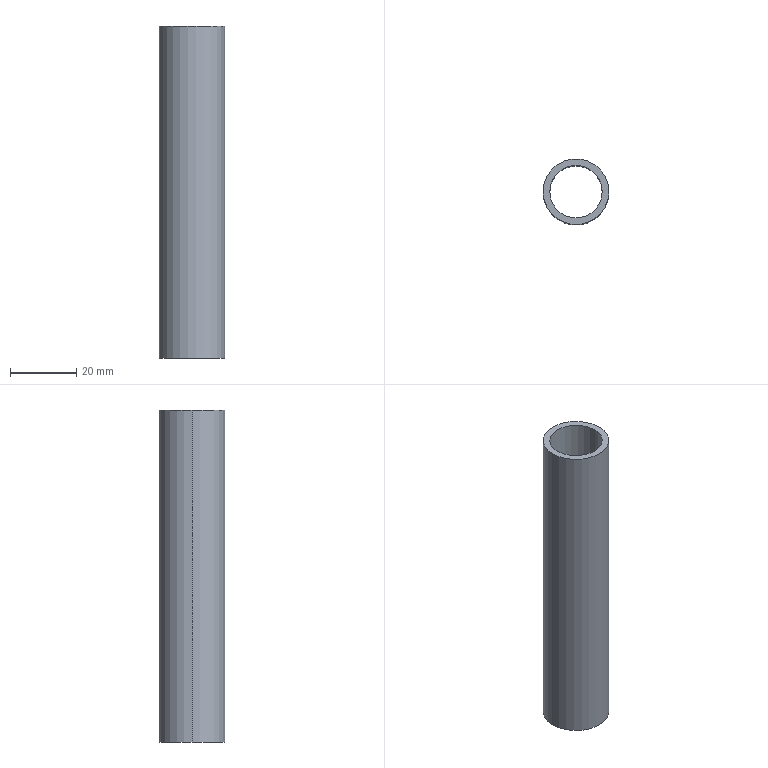Part | STEP file | 51E-01159JG10 | 1 solid | 6 faces | box 19.8 x 19.8 x 100 mm | volume 11184 mm3 | cylinder 4 | plane 2 | commonest cylinder face diameters 15.8 x2 19.8 x2
STEP:
#1=CARTESIAN_POINT('',(-7.9,0.,100.));
#2=VERTEX_POINT('',#1);
#3=CARTESIAN_POINT('',(7.9,0.,100.));
#4=VERTEX_POINT('',#3);
#5=CARTESIAN_POINT('',(0.,0.,100.));
#6=DIRECTION('',(0.,0.,-1.));
#7=AXIS2_PLACEMENT_3D('',#5,#6,$);
#8=CIRCLE('',#7,7.9);
#9=EDGE_CURVE('',#2,#4,#8,.F.);
#10=ORIENTED_EDGE('',*,*,#9,.T.);
#11=CARTESIAN_POINT('',(7.9,0.,0.));
#12=VERTEX_POINT('',#11);
#13=CARTESIAN_POINT('',(7.9,0.,100.));
#14=DIRECTION('',(0.,0.,-1.));
#15=VECTOR('',#14,1.);
#16=LINE('',#13,#15);
#17=EDGE_CURVE('',#4,#12,#16,.T.);
#18=ORIENTED_EDGE('',*,*,#17,.T.);
#19=CARTESIAN_POINT('',(-7.9,0.,0.));
#20=VERTEX_POINT('',#19);
#21=CARTESIAN_POINT('',(0.,0.,0.));
#22=DIRECTION('',(0.,0.,-1.));
#23=AXIS2_PLACEMENT_3D('',#21,#22,$);
#24=CIRCLE('',#23,7.9);
#25=EDGE_CURVE('',#20,#12,#24,.F.);
#26=ORIENTED_EDGE('',*,*,#25,.F.);
#27=CARTESIAN_POINT('',(-7.9,0.,100.));
#28=DIRECTION('',(0.,0.,-1.));
#29=VECTOR('',#28,1.);
#30=LINE('',#27,#29);
#31=EDGE_CURVE('',#2,#20,#30,.T.);
#32=ORIENTED_EDGE('',*,*,#31,.F.);
#33=EDGE_LOOP('',(#10,#18,#26,#32));
#34=FACE_OUTER_BOUND('',#33,.T.);
#35=CARTESIAN_POINT('',(0.,0.,100.));
#36=DIRECTION('',(0.,0.,-1.));
#37=DIRECTION('',(1.,0.,0.));
#38=AXIS2_PLACEMENT_3D('',#35,#36,#37);
#39=CYLINDRICAL_SURFACE('',#38,7.9);
#40=ADVANCED_FACE('',(#34),#39,.F.);
#41=CARTESIAN_POINT('',(-9.9,0.,100.));
#42=VERTEX_POINT('',#41);
#43=CARTESIAN_POINT('',(9.9,0.,100.));
#44=VERTEX_POINT('',#43);
#45=CARTESIAN_POINT('',(0.,0.,100.));
#46=DIRECTION('',(0.,0.,1.));
#47=AXIS2_PLACEMENT_3D('',#45,#46,$);
#48=CIRCLE('',#47,9.9);
#49=EDGE_CURVE('',#42,#44,#48,.T.);
#50=ORIENTED_EDGE('',*,*,#49,.T.);
#51=CARTESIAN_POINT('',(0.,0.,100.));
#52=DIRECTION('',(0.,0.,1.));
#53=AXIS2_PLACEMENT_3D('',#51,#52,$);
#54=CIRCLE('',#53,9.9);
#55=EDGE_CURVE('',#44,#42,#54,.T.);
#56=ORIENTED_EDGE('',*,*,#55,.T.);
#57=EDGE_LOOP('',(#50,#56));
#58=FACE_OUTER_BOUND('',#57,.T.);
#59=ORIENTED_EDGE('',*,*,#9,.F.);
#60=CARTESIAN_POINT('',(0.,0.,100.));
#61=DIRECTION('',(0.,0.,1.));
#62=AXIS2_PLACEMENT_3D('',#60,#61,$);
#63=CIRCLE('',#62,7.9);
#64=EDGE_CURVE('',#4,#2,#63,.T.);
#65=ORIENTED_EDGE('',*,*,#64,.F.);
#66=EDGE_LOOP('',(#59,#65));
#67=FACE_BOUND('',#66,.T.);
#68=CARTESIAN_POINT('',(0.,0.,100.));
#69=DIRECTION('',(0.,0.,1.));
#70=DIRECTION('',(1.,0.,0.));
#71=AXIS2_PLACEMENT_3D('',#68,#69,#70);
#72=PLANE('',#71);
#73=ADVANCED_FACE('',(#58,#67),#72,.T.);
#74=ORIENTED_EDGE('',*,*,#17,.F.);
#75=ORIENTED_EDGE('',*,*,#64,.T.);
#76=ORIENTED_EDGE('',*,*,#31,.T.);
#77=CARTESIAN_POINT('',(0.,0.,0.));
#78=DIRECTION('',(0.,0.,-1.));
#79=AXIS2_PLACEMENT_3D('',#77,#78,$);
#80=CIRCLE('',#79,7.9);
#81=EDGE_CURVE('',#12,#20,#80,.F.);
#82=ORIENTED_EDGE('',*,*,#81,.F.);
#83=EDGE_LOOP('',(#74,#75,#76,#82));
#84=FACE_OUTER_BOUND('',#83,.T.);
#85=CARTESIAN_POINT('',(0.,0.,100.));
#86=DIRECTION('',(0.,0.,-1.));
#87=DIRECTION('',(-1.,0.,0.));
#88=AXIS2_PLACEMENT_3D('',#85,#86,#87);
#89=CYLINDRICAL_SURFACE('',#88,7.9);
#90=ADVANCED_FACE('',(#84),#89,.F.);
#91=CARTESIAN_POINT('',(-9.9,0.,0.));
#92=VERTEX_POINT('',#91);
#93=CARTESIAN_POINT('',(9.9,0.,0.));
#94=VERTEX_POINT('',#93);
#95=CARTESIAN_POINT('',(0.,0.,0.));
#96=DIRECTION('',(0.,0.,1.));
#97=AXIS2_PLACEMENT_3D('',#95,#96,$);
#98=CIRCLE('',#97,9.9);
#99=EDGE_CURVE('',#92,#94,#98,.T.);
#100=ORIENTED_EDGE('',*,*,#99,.F.);
#101=CARTESIAN_POINT('',(0.,0.,0.));
#102=DIRECTION('',(0.,0.,1.));
#103=AXIS2_PLACEMENT_3D('',#101,#102,$);
#104=CIRCLE('',#103,9.9);
#105=EDGE_CURVE('',#94,#92,#104,.T.);
#106=ORIENTED_EDGE('',*,*,#105,.F.);
#107=EDGE_LOOP('',(#100,#106));
#108=FACE_OUTER_BOUND('',#107,.T.);
#109=ORIENTED_EDGE('',*,*,#25,.T.);
#110=ORIENTED_EDGE('',*,*,#81,.T.);
#111=EDGE_LOOP('',(#109,#110));
#112=FACE_BOUND('',#111,.T.);
#113=CARTESIAN_POINT('',(0.,0.,0.));
#114=DIRECTION('',(0.,0.,1.));
#115=DIRECTION('',(1.,0.,0.));
#116=AXIS2_PLACEMENT_3D('',#113,#114,#115);
#117=PLANE('',#116);
#118=ADVANCED_FACE('',(#108,#112),#117,.F.);
#119=CARTESIAN_POINT('',(9.9,0.,100.));
#120=DIRECTION('',(0.,0.,-1.));
#121=VECTOR('',#120,1.);
#122=LINE('',#119,#121);
#123=EDGE_CURVE('',#44,#94,#122,.T.);
#124=ORIENTED_EDGE('',*,*,#123,.F.);
#125=ORIENTED_EDGE('',*,*,#49,.F.);
#126=CARTESIAN_POINT('',(-9.9,0.,100.));
#127=DIRECTION('',(0.,0.,-1.));
#128=VECTOR('',#127,1.);
#129=LINE('',#126,#128);
#130=EDGE_CURVE('',#42,#92,#129,.T.);
#131=ORIENTED_EDGE('',*,*,#130,.T.);
#132=ORIENTED_EDGE('',*,*,#99,.T.);
#133=EDGE_LOOP('',(#124,#125,#131,#132));
#134=FACE_OUTER_BOUND('',#133,.T.);
#135=CARTESIAN_POINT('',(0.,0.,100.));
#136=DIRECTION('',(0.,0.,-1.));
#137=DIRECTION('',(1.,0.,0.));
#138=AXIS2_PLACEMENT_3D('',#135,#136,#137);
#139=CYLINDRICAL_SURFACE('',#138,9.9);
#140=ADVANCED_FACE('',(#134),#139,.T.);
#141=ORIENTED_EDGE('',*,*,#55,.F.);
#142=ORIENTED_EDGE('',*,*,#123,.T.);
#143=ORIENTED_EDGE('',*,*,#105,.T.);
#144=ORIENTED_EDGE('',*,*,#130,.F.);
#145=EDGE_LOOP('',(#141,#142,#143,#144));
#146=FACE_OUTER_BOUND('',#145,.T.);
#147=CARTESIAN_POINT('',(0.,0.,100.));
#148=DIRECTION('',(0.,0.,-1.));
#149=DIRECTION('',(-1.,0.,0.));
#150=AXIS2_PLACEMENT_3D('',#147,#148,#149);
#151=CYLINDRICAL_SURFACE('',#150,9.9);
#152=ADVANCED_FACE('',(#146),#151,.T.);
#153=CLOSED_SHELL('',(#40,#73,#90,#118,#140,#152));
#154=MANIFOLD_SOLID_BREP('',#153);
#155=(LENGTH_UNIT()NAMED_UNIT(*)SI_UNIT(.MILLI.,.METRE.));
#156=UNCERTAINTY_MEASURE_WITH_UNIT(LENGTH_MEASURE(0.005),#155,'','');
#157=(NAMED_UNIT(*)PLANE_ANGLE_UNIT()SI_UNIT($,.RADIAN.));
#158=(NAMED_UNIT(*)SI_UNIT($,.STERADIAN.)SOLID_ANGLE_UNIT());
#159=(GEOMETRIC_REPRESENTATION_CONTEXT(3)GLOBAL_UNCERTAINTY_ASSIGNED_CONTEXT((#156))GLOBAL_UNIT_ASSIGNED_CONTEXT((#155,#157,#158))REPRESENTATION_CONTEXT('',''));
#160=ADVANCED_BREP_SHAPE_REPRESENTATION('',(#154),#159);